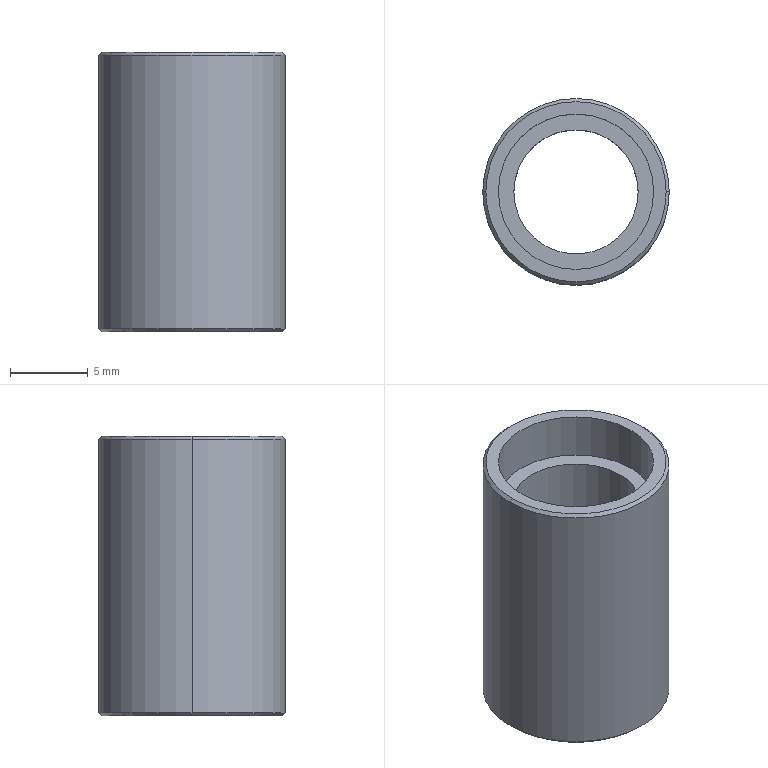Part | SolidWorks | features Chamfer 1, Extrusion 1, ICE 1, MirrorPattern 1 | 1 solid | 16 faces | box 12 x 12 x 18 mm | volume 959.836 mm3 | cylinder 8 | cone 4 | plane 4 | commonest cylinder face diameters 10 x4 8 x2 12 x2
STEP:
#1=CARTESIAN_POINT('',(5.8,0.,9.));
#2=VERTEX_POINT('',#1);
#3=CARTESIAN_POINT('',(-5.8,0.,9.));
#4=VERTEX_POINT('',#3);
#5=CARTESIAN_POINT('',(0.,0.,9.));
#6=DIRECTION('',(0.,0.,1.));
#7=DIRECTION('',(1.,0.,0.));
#8=AXIS2_PLACEMENT_3D('',#5,#6,#7);
#9=CIRCLE('',#8,5.8);
#10=EDGE_CURVE('',#2,#4,#9,.T.);
#11=ORIENTED_EDGE('',*,*,#10,.F.);
#12=CARTESIAN_POINT('',(6.,0.,8.8));
#13=VERTEX_POINT('',#12);
#14=CARTESIAN_POINT('',(5.8,0.,9.));
#15=DIRECTION('',(0.7071,0.,-0.7071));
#16=VECTOR('',#15,1000.);
#17=LINE('',#14,#16);
#18=EDGE_CURVE('',#2,#13,#17,.T.);
#19=ORIENTED_EDGE('',*,*,#18,.T.);
#20=CARTESIAN_POINT('',(-6.,0.,8.8));
#21=VERTEX_POINT('',#20);
#22=CARTESIAN_POINT('',(0.,0.,8.8));
#23=DIRECTION('',(0.,0.,-1.));
#24=DIRECTION('',(1.,0.,0.));
#25=AXIS2_PLACEMENT_3D('',#22,#23,#24);
#26=CIRCLE('',#25,6.);
#27=EDGE_CURVE('',#21,#13,#26,.T.);
#28=ORIENTED_EDGE('',*,*,#27,.F.);
#29=CARTESIAN_POINT('',(-5.8,0.,9.));
#30=DIRECTION('',(-0.7071,0.,-0.7071));
#31=VECTOR('',#30,1000.);
#32=LINE('',#29,#31);
#33=EDGE_CURVE('',#4,#21,#32,.T.);
#34=ORIENTED_EDGE('',*,*,#33,.F.);
#35=EDGE_LOOP('',(#11,#19,#28,#34));
#36=FACE_OUTER_BOUND('',#35,.T.);
#37=CARTESIAN_POINT('',(0.,0.,9.));
#38=DIRECTION('',(0.,0.,-1.));
#39=DIRECTION('',(-1.,0.,0.));
#40=AXIS2_PLACEMENT_3D('',#37,#38,#39);
#41=CONICAL_SURFACE('',#40,5.8,0.7854);
#42=ADVANCED_FACE('',(#36),#41,.T.);
#43=CARTESIAN_POINT('',(-5.8,0.,-9.));
#44=VERTEX_POINT('',#43);
#45=CARTESIAN_POINT('',(5.8,0.,-9.));
#46=VERTEX_POINT('',#45);
#47=CARTESIAN_POINT('',(0.,0.,-9.));
#48=DIRECTION('',(0.,0.,-1.));
#49=DIRECTION('',(1.,0.,0.));
#50=AXIS2_PLACEMENT_3D('',#47,#48,#49);
#51=CIRCLE('',#50,5.8);
#52=EDGE_CURVE('',#44,#46,#51,.T.);
#53=ORIENTED_EDGE('',*,*,#52,.F.);
#54=CARTESIAN_POINT('',(-6.,0.,-8.8));
#55=VERTEX_POINT('',#54);
#56=CARTESIAN_POINT('',(-6.,0.,-8.8));
#57=DIRECTION('',(-0.7071,0.,0.7071));
#58=VECTOR('',#57,1000.);
#59=LINE('',#56,#58);
#60=EDGE_CURVE('',#44,#55,#59,.T.);
#61=ORIENTED_EDGE('',*,*,#60,.T.);
#62=CARTESIAN_POINT('',(6.,0.,-8.8));
#63=VERTEX_POINT('',#62);
#64=CARTESIAN_POINT('',(0.,0.,-8.8));
#65=DIRECTION('',(0.,0.,1.));
#66=DIRECTION('',(1.,0.,0.));
#67=AXIS2_PLACEMENT_3D('',#64,#65,#66);
#68=CIRCLE('',#67,6.);
#69=EDGE_CURVE('',#63,#55,#68,.T.);
#70=ORIENTED_EDGE('',*,*,#69,.F.);
#71=CARTESIAN_POINT('',(6.,0.,-8.8));
#72=DIRECTION('',(0.7071,0.,0.7071));
#73=VECTOR('',#72,1000.);
#74=LINE('',#71,#73);
#75=EDGE_CURVE('',#46,#63,#74,.T.);
#76=ORIENTED_EDGE('',*,*,#75,.F.);
#77=EDGE_LOOP('',(#53,#61,#70,#76));
#78=FACE_OUTER_BOUND('',#77,.T.);
#79=CARTESIAN_POINT('',(0.,0.,-8.8));
#80=DIRECTION('',(0.,0.,1.));
#81=DIRECTION('',(1.,0.,0.));
#82=AXIS2_PLACEMENT_3D('',#79,#80,#81);
#83=CONICAL_SURFACE('',#82,6.,0.7854);
#84=ADVANCED_FACE('',(#78),#83,.T.);
#85=CARTESIAN_POINT('',(-5.,0.,-6.));
#86=VERTEX_POINT('',#85);
#87=CARTESIAN_POINT('',(5.,0.,-6.));
#88=VERTEX_POINT('',#87);
#89=CARTESIAN_POINT('',(0.,0.,-6.));
#90=DIRECTION('',(0.,0.,1.));
#91=DIRECTION('',(1.,0.,0.));
#92=AXIS2_PLACEMENT_3D('',#89,#90,#91);
#93=CIRCLE('',#92,5.);
#94=EDGE_CURVE('',#86,#88,#93,.T.);
#95=ORIENTED_EDGE('',*,*,#94,.T.);
#96=CARTESIAN_POINT('',(5.,0.,-9.));
#97=VERTEX_POINT('',#96);
#98=CARTESIAN_POINT('',(5.,0.,-6.));
#99=DIRECTION('',(0.,0.,-1.));
#100=VECTOR('',#99,1000.);
#101=LINE('',#98,#100);
#102=EDGE_CURVE('',#88,#97,#101,.T.);
#103=ORIENTED_EDGE('',*,*,#102,.T.);
#104=CARTESIAN_POINT('',(-5.,0.,-9.));
#105=VERTEX_POINT('',#104);
#106=CARTESIAN_POINT('',(0.,0.,-9.));
#107=DIRECTION('',(0.,0.,1.));
#108=DIRECTION('',(1.,0.,0.));
#109=AXIS2_PLACEMENT_3D('',#106,#107,#108);
#110=CIRCLE('',#109,5.);
#111=EDGE_CURVE('',#105,#97,#110,.T.);
#112=ORIENTED_EDGE('',*,*,#111,.F.);
#113=CARTESIAN_POINT('',(-5.,0.,-6.));
#114=DIRECTION('',(0.,0.,-1.));
#115=VECTOR('',#114,1000.);
#116=LINE('',#113,#115);
#117=EDGE_CURVE('',#86,#105,#116,.T.);
#118=ORIENTED_EDGE('',*,*,#117,.F.);
#119=EDGE_LOOP('',(#95,#103,#112,#118));
#120=FACE_OUTER_BOUND('',#119,.T.);
#121=CARTESIAN_POINT('',(0.,0.,-6.));
#122=DIRECTION('',(0.,0.,-1.));
#123=DIRECTION('',(-1.,0.,0.));
#124=AXIS2_PLACEMENT_3D('',#121,#122,#123);
#125=CYLINDRICAL_SURFACE('',#124,5.);
#126=ADVANCED_FACE('',(#120),#125,.F.);
#127=CARTESIAN_POINT('',(-5.,0.,6.));
#128=VERTEX_POINT('',#127);
#129=CARTESIAN_POINT('',(5.,0.,6.));
#130=VERTEX_POINT('',#129);
#131=CARTESIAN_POINT('',(0.,0.,6.));
#132=DIRECTION('',(0.,0.,1.));
#133=DIRECTION('',(1.,0.,0.));
#134=AXIS2_PLACEMENT_3D('',#131,#132,#133);
#135=CIRCLE('',#134,5.);
#136=EDGE_CURVE('',#128,#130,#135,.T.);
#137=ORIENTED_EDGE('',*,*,#136,.F.);
#138=CARTESIAN_POINT('',(-5.,0.,9.));
#139=VERTEX_POINT('',#138);
#140=CARTESIAN_POINT('',(-5.,0.,6.));
#141=DIRECTION('',(0.,0.,1.));
#142=VECTOR('',#141,1000.);
#143=LINE('',#140,#142);
#144=EDGE_CURVE('',#128,#139,#143,.T.);
#145=ORIENTED_EDGE('',*,*,#144,.T.);
#146=CARTESIAN_POINT('',(5.,0.,9.));
#147=VERTEX_POINT('',#146);
#148=CARTESIAN_POINT('',(0.,0.,9.));
#149=DIRECTION('',(0.,0.,1.));
#150=DIRECTION('',(1.,0.,0.));
#151=AXIS2_PLACEMENT_3D('',#148,#149,#150);
#152=CIRCLE('',#151,5.);
#153=EDGE_CURVE('',#139,#147,#152,.T.);
#154=ORIENTED_EDGE('',*,*,#153,.T.);
#155=CARTESIAN_POINT('',(5.,0.,6.));
#156=DIRECTION('',(0.,0.,1.));
#157=VECTOR('',#156,1000.);
#158=LINE('',#155,#157);
#159=EDGE_CURVE('',#130,#147,#158,.T.);
#160=ORIENTED_EDGE('',*,*,#159,.F.);
#161=EDGE_LOOP('',(#137,#145,#154,#160));
#162=FACE_OUTER_BOUND('',#161,.T.);
#163=CARTESIAN_POINT('',(0.,0.,6.));
#164=DIRECTION('',(0.,0.,1.));
#165=DIRECTION('',(1.,0.,0.));
#166=AXIS2_PLACEMENT_3D('',#163,#164,#165);
#167=CYLINDRICAL_SURFACE('',#166,5.);
#168=ADVANCED_FACE('',(#162),#167,.F.);
#169=ORIENTED_EDGE('',*,*,#27,.T.);
#170=CARTESIAN_POINT('',(6.,0.,9.));
#171=DIRECTION('',(0.,0.,-1.));
#172=VECTOR('',#171,1000.);
#173=LINE('',#170,#172);
#174=EDGE_CURVE('',#13,#63,#173,.T.);
#175=ORIENTED_EDGE('',*,*,#174,.T.);
#176=ORIENTED_EDGE('',*,*,#69,.T.);
#177=CARTESIAN_POINT('',(-6.,0.,9.));
#178=DIRECTION('',(0.,0.,-1.));
#179=VECTOR('',#178,1000.);
#180=LINE('',#177,#179);
#181=EDGE_CURVE('',#21,#55,#180,.T.);
#182=ORIENTED_EDGE('',*,*,#181,.F.);
#183=EDGE_LOOP('',(#169,#175,#176,#182));
#184=FACE_OUTER_BOUND('',#183,.T.);
#185=CARTESIAN_POINT('',(0.,0.,9.));
#186=DIRECTION('',(0.,0.,-1.));
#187=DIRECTION('',(-1.,0.,0.));
#188=AXIS2_PLACEMENT_3D('',#185,#186,#187);
#189=CYLINDRICAL_SURFACE('',#188,6.);
#190=ADVANCED_FACE('',(#184),#189,.T.);
#191=CARTESIAN_POINT('',(-4.,0.,6.));
#192=VERTEX_POINT('',#191);
#193=CARTESIAN_POINT('',(4.,0.,6.));
#194=VERTEX_POINT('',#193);
#195=CARTESIAN_POINT('',(0.,0.,6.));
#196=DIRECTION('',(0.,0.,1.));
#197=DIRECTION('',(1.,0.,0.));
#198=AXIS2_PLACEMENT_3D('',#195,#196,#197);
#199=CIRCLE('',#198,4.);
#200=EDGE_CURVE('',#192,#194,#199,.T.);
#201=ORIENTED_EDGE('',*,*,#200,.T.);
#202=CARTESIAN_POINT('',(4.,0.,-6.));
#203=VERTEX_POINT('',#202);
#204=CARTESIAN_POINT('',(4.,0.,9.));
#205=DIRECTION('',(0.,0.,-1.));
#206=VECTOR('',#205,1000.);
#207=LINE('',#204,#206);
#208=EDGE_CURVE('',#194,#203,#207,.T.);
#209=ORIENTED_EDGE('',*,*,#208,.T.);
#210=CARTESIAN_POINT('',(-4.,0.,-6.));
#211=VERTEX_POINT('',#210);
#212=CARTESIAN_POINT('',(0.,0.,-6.));
#213=DIRECTION('',(0.,0.,-1.));
#214=DIRECTION('',(-1.,0.,0.));
#215=AXIS2_PLACEMENT_3D('',#212,#213,#214);
#216=CIRCLE('',#215,4.);
#217=EDGE_CURVE('',#203,#211,#216,.T.);
#218=ORIENTED_EDGE('',*,*,#217,.T.);
#219=CARTESIAN_POINT('',(-4.,0.,9.));
#220=DIRECTION('',(0.,0.,-1.));
#221=VECTOR('',#220,1000.);
#222=LINE('',#219,#221);
#223=EDGE_CURVE('',#192,#211,#222,.T.);
#224=ORIENTED_EDGE('',*,*,#223,.F.);
#225=EDGE_LOOP('',(#201,#209,#218,#224));
#226=FACE_OUTER_BOUND('',#225,.T.);
#227=CARTESIAN_POINT('',(0.,0.,9.));
#228=DIRECTION('',(0.,0.,-1.));
#229=DIRECTION('',(-1.,0.,0.));
#230=AXIS2_PLACEMENT_3D('',#227,#228,#229);
#231=CYLINDRICAL_SURFACE('',#230,4.);
#232=ADVANCED_FACE('',(#226),#231,.F.);
#233=ORIENTED_EDGE('',*,*,#208,.F.);
#234=CARTESIAN_POINT('',(0.,0.,6.));
#235=DIRECTION('',(0.,0.,1.));
#236=DIRECTION('',(1.,0.,0.));
#237=AXIS2_PLACEMENT_3D('',#234,#235,#236);
#238=CIRCLE('',#237,4.);
#239=EDGE_CURVE('',#194,#192,#238,.T.);
#240=ORIENTED_EDGE('',*,*,#239,.T.);
#241=ORIENTED_EDGE('',*,*,#223,.T.);
#242=CARTESIAN_POINT('',(0.,0.,-6.));
#243=DIRECTION('',(0.,0.,-1.));
#244=DIRECTION('',(-1.,0.,0.));
#245=AXIS2_PLACEMENT_3D('',#242,#243,#244);
#246=CIRCLE('',#245,4.);
#247=EDGE_CURVE('',#211,#203,#246,.T.);
#248=ORIENTED_EDGE('',*,*,#247,.T.);
#249=EDGE_LOOP('',(#233,#240,#241,#248));
#250=FACE_OUTER_BOUND('',#249,.T.);
#251=CARTESIAN_POINT('',(0.,0.,9.));
#252=DIRECTION('',(0.,0.,-1.));
#253=DIRECTION('',(-1.,0.,0.));
#254=AXIS2_PLACEMENT_3D('',#251,#252,#253);
#255=CYLINDRICAL_SURFACE('',#254,4.);
#256=ADVANCED_FACE('',(#250),#255,.F.);
#257=CARTESIAN_POINT('',(0.,0.,-9.));
#258=DIRECTION('',(0.,0.,-1.));
#259=DIRECTION('',(1.,0.,0.));
#260=AXIS2_PLACEMENT_3D('',#257,#258,#259);
#261=CIRCLE('',#260,5.8);
#262=EDGE_CURVE('',#46,#44,#261,.T.);
#263=ORIENTED_EDGE('',*,*,#262,.T.);
#264=ORIENTED_EDGE('',*,*,#52,.T.);
#265=EDGE_LOOP('',(#263,#264));
#266=FACE_OUTER_BOUND('',#265,.T.);
#267=ORIENTED_EDGE('',*,*,#111,.T.);
#268=CARTESIAN_POINT('',(0.,0.,-9.));
#269=DIRECTION('',(0.,0.,1.));
#270=DIRECTION('',(1.,0.,0.));
#271=AXIS2_PLACEMENT_3D('',#268,#269,#270);
#272=CIRCLE('',#271,5.);
#273=EDGE_CURVE('',#97,#105,#272,.T.);
#274=ORIENTED_EDGE('',*,*,#273,.T.);
#275=EDGE_LOOP('',(#267,#274));
#276=FACE_BOUND('',#275,.T.);
#277=CARTESIAN_POINT('',(0.,0.,-9.));
#278=DIRECTION('',(0.,0.,1.));
#279=DIRECTION('',(1.,0.,0.));
#280=AXIS2_PLACEMENT_3D('',#277,#278,#279);
#281=PLANE('',#280);
#282=ADVANCED_FACE('',(#266,#276),#281,.F.);
#283=CARTESIAN_POINT('',(0.,0.,9.));
#284=DIRECTION('',(0.,0.,1.));
#285=DIRECTION('',(1.,0.,0.));
#286=AXIS2_PLACEMENT_3D('',#283,#284,#285);
#287=CIRCLE('',#286,5.8);
#288=EDGE_CURVE('',#4,#2,#287,.T.);
#289=ORIENTED_EDGE('',*,*,#288,.T.);
#290=ORIENTED_EDGE('',*,*,#10,.T.);
#291=EDGE_LOOP('',(#289,#290));
#292=FACE_OUTER_BOUND('',#291,.T.);
#293=CARTESIAN_POINT('',(0.,0.,9.));
#294=DIRECTION('',(0.,0.,1.));
#295=DIRECTION('',(1.,0.,0.));
#296=AXIS2_PLACEMENT_3D('',#293,#294,#295);
#297=CIRCLE('',#296,5.);
#298=EDGE_CURVE('',#147,#139,#297,.T.);
#299=ORIENTED_EDGE('',*,*,#298,.F.);
#300=ORIENTED_EDGE('',*,*,#153,.F.);
#301=EDGE_LOOP('',(#299,#300));
#302=FACE_BOUND('',#301,.T.);
#303=CARTESIAN_POINT('',(0.,0.,9.));
#304=DIRECTION('',(0.,0.,1.));
#305=DIRECTION('',(1.,0.,0.));
#306=AXIS2_PLACEMENT_3D('',#303,#304,#305);
#307=PLANE('',#306);
#308=ADVANCED_FACE('',(#292,#302),#307,.T.);
#309=ORIENTED_EDGE('',*,*,#174,.F.);
#310=CARTESIAN_POINT('',(0.,0.,8.8));
#311=DIRECTION('',(0.,0.,-1.));
#312=DIRECTION('',(1.,0.,0.));
#313=AXIS2_PLACEMENT_3D('',#310,#311,#312);
#314=CIRCLE('',#313,6.);
#315=EDGE_CURVE('',#13,#21,#314,.T.);
#316=ORIENTED_EDGE('',*,*,#315,.T.);
#317=ORIENTED_EDGE('',*,*,#181,.T.);
#318=CARTESIAN_POINT('',(0.,0.,-8.8));
#319=DIRECTION('',(0.,0.,1.));
#320=DIRECTION('',(1.,0.,0.));
#321=AXIS2_PLACEMENT_3D('',#318,#319,#320);
#322=CIRCLE('',#321,6.);
#323=EDGE_CURVE('',#55,#63,#322,.T.);
#324=ORIENTED_EDGE('',*,*,#323,.T.);
#325=EDGE_LOOP('',(#309,#316,#317,#324));
#326=FACE_OUTER_BOUND('',#325,.T.);
#327=CARTESIAN_POINT('',(0.,0.,9.));
#328=DIRECTION('',(0.,0.,-1.));
#329=DIRECTION('',(-1.,0.,0.));
#330=AXIS2_PLACEMENT_3D('',#327,#328,#329);
#331=CYLINDRICAL_SURFACE('',#330,6.);
#332=ADVANCED_FACE('',(#326),#331,.T.);
#333=ORIENTED_EDGE('',*,*,#144,.F.);
#334=CARTESIAN_POINT('',(0.,0.,6.));
#335=DIRECTION('',(0.,0.,1.));
#336=DIRECTION('',(1.,0.,0.));
#337=AXIS2_PLACEMENT_3D('',#334,#335,#336);
#338=CIRCLE('',#337,5.);
#339=EDGE_CURVE('',#130,#128,#338,.T.);
#340=ORIENTED_EDGE('',*,*,#339,.F.);
#341=ORIENTED_EDGE('',*,*,#159,.T.);
#342=ORIENTED_EDGE('',*,*,#298,.T.);
#343=EDGE_LOOP('',(#333,#340,#341,#342));
#344=FACE_OUTER_BOUND('',#343,.T.);
#345=CARTESIAN_POINT('',(0.,0.,6.));
#346=DIRECTION('',(0.,0.,1.));
#347=DIRECTION('',(1.,0.,0.));
#348=AXIS2_PLACEMENT_3D('',#345,#346,#347);
#349=CYLINDRICAL_SURFACE('',#348,5.);
#350=ADVANCED_FACE('',(#344),#349,.F.);
#351=ORIENTED_EDGE('',*,*,#200,.F.);
#352=ORIENTED_EDGE('',*,*,#239,.F.);
#353=EDGE_LOOP('',(#351,#352));
#354=FACE_BOUND('',#353,.T.);
#355=ORIENTED_EDGE('',*,*,#339,.T.);
#356=ORIENTED_EDGE('',*,*,#136,.T.);
#357=EDGE_LOOP('',(#355,#356));
#358=FACE_OUTER_BOUND('',#357,.T.);
#359=CARTESIAN_POINT('',(0.,0.,6.));
#360=DIRECTION('',(0.,0.,1.));
#361=DIRECTION('',(1.,0.,0.));
#362=AXIS2_PLACEMENT_3D('',#359,#360,#361);
#363=PLANE('',#362);
#364=ADVANCED_FACE('',(#354,#358),#363,.T.);
#365=ORIENTED_EDGE('',*,*,#102,.F.);
#366=CARTESIAN_POINT('',(0.,0.,-6.));
#367=DIRECTION('',(0.,0.,1.));
#368=DIRECTION('',(1.,0.,0.));
#369=AXIS2_PLACEMENT_3D('',#366,#367,#368);
#370=CIRCLE('',#369,5.);
#371=EDGE_CURVE('',#88,#86,#370,.T.);
#372=ORIENTED_EDGE('',*,*,#371,.T.);
#373=ORIENTED_EDGE('',*,*,#117,.T.);
#374=ORIENTED_EDGE('',*,*,#273,.F.);
#375=EDGE_LOOP('',(#365,#372,#373,#374));
#376=FACE_OUTER_BOUND('',#375,.T.);
#377=CARTESIAN_POINT('',(0.,0.,-6.));
#378=DIRECTION('',(0.,0.,-1.));
#379=DIRECTION('',(-1.,0.,0.));
#380=AXIS2_PLACEMENT_3D('',#377,#378,#379);
#381=CYLINDRICAL_SURFACE('',#380,5.);
#382=ADVANCED_FACE('',(#376),#381,.F.);
#383=ORIENTED_EDGE('',*,*,#247,.F.);
#384=ORIENTED_EDGE('',*,*,#217,.F.);
#385=EDGE_LOOP('',(#383,#384));
#386=FACE_BOUND('',#385,.T.);
#387=ORIENTED_EDGE('',*,*,#94,.F.);
#388=ORIENTED_EDGE('',*,*,#371,.F.);
#389=EDGE_LOOP('',(#387,#388));
#390=FACE_OUTER_BOUND('',#389,.T.);
#391=CARTESIAN_POINT('',(0.,0.,-6.));
#392=DIRECTION('',(0.,0.,-1.));
#393=DIRECTION('',(1.,0.,0.));
#394=AXIS2_PLACEMENT_3D('',#391,#392,#393);
#395=PLANE('',#394);
#396=ADVANCED_FACE('',(#386,#390),#395,.T.);
#397=ORIENTED_EDGE('',*,*,#60,.F.);
#398=ORIENTED_EDGE('',*,*,#262,.F.);
#399=ORIENTED_EDGE('',*,*,#75,.T.);
#400=ORIENTED_EDGE('',*,*,#323,.F.);
#401=EDGE_LOOP('',(#397,#398,#399,#400));
#402=FACE_OUTER_BOUND('',#401,.T.);
#403=CARTESIAN_POINT('',(0.,0.,-8.8));
#404=DIRECTION('',(0.,0.,1.));
#405=DIRECTION('',(1.,0.,0.));
#406=AXIS2_PLACEMENT_3D('',#403,#404,#405);
#407=CONICAL_SURFACE('',#406,6.,0.7854);
#408=ADVANCED_FACE('',(#402),#407,.T.);
#409=ORIENTED_EDGE('',*,*,#18,.F.);
#410=ORIENTED_EDGE('',*,*,#288,.F.);
#411=ORIENTED_EDGE('',*,*,#33,.T.);
#412=ORIENTED_EDGE('',*,*,#315,.F.);
#413=EDGE_LOOP('',(#409,#410,#411,#412));
#414=FACE_OUTER_BOUND('',#413,.T.);
#415=CARTESIAN_POINT('',(0.,0.,9.));
#416=DIRECTION('',(0.,0.,-1.));
#417=DIRECTION('',(-1.,0.,0.));
#418=AXIS2_PLACEMENT_3D('',#415,#416,#417);
#419=CONICAL_SURFACE('',#418,5.8,0.7854);
#420=ADVANCED_FACE('',(#414),#419,.T.);
#421=CLOSED_SHELL('',(#42,#84,#126,#168,#190,#232,#256,#282,#308,#332,#350,#364,#382,#396,#408,#420));
#422=MANIFOLD_SOLID_BREP('',#421);
#423=CARTESIAN_POINT('',(0.,0.,0.));
#424=DIRECTION('',(0.,0.,1.));
#425=DIRECTION('',(1.,0.,0.));
#426=AXIS2_PLACEMENT_3D('',#423,#424,#425);
#427=(LENGTH_UNIT()NAMED_UNIT(*)SI_UNIT(.MILLI.,.METRE.));
#428=UNCERTAINTY_MEASURE_WITH_UNIT(LENGTH_MEASURE(0.00001),#427,'','');
#429=(NAMED_UNIT(*)PLANE_ANGLE_UNIT()SI_UNIT($,.RADIAN.));
#430=(NAMED_UNIT(*)SI_UNIT($,.STERADIAN.)SOLID_ANGLE_UNIT());
#431=(GEOMETRIC_REPRESENTATION_CONTEXT(3)GLOBAL_UNCERTAINTY_ASSIGNED_CONTEXT((#428))GLOBAL_UNIT_ASSIGNED_CONTEXT((#427,#429,#430))REPRESENTATION_CONTEXT('',''));
#432=ADVANCED_BREP_SHAPE_REPRESENTATION('',(#422,#426),#431);